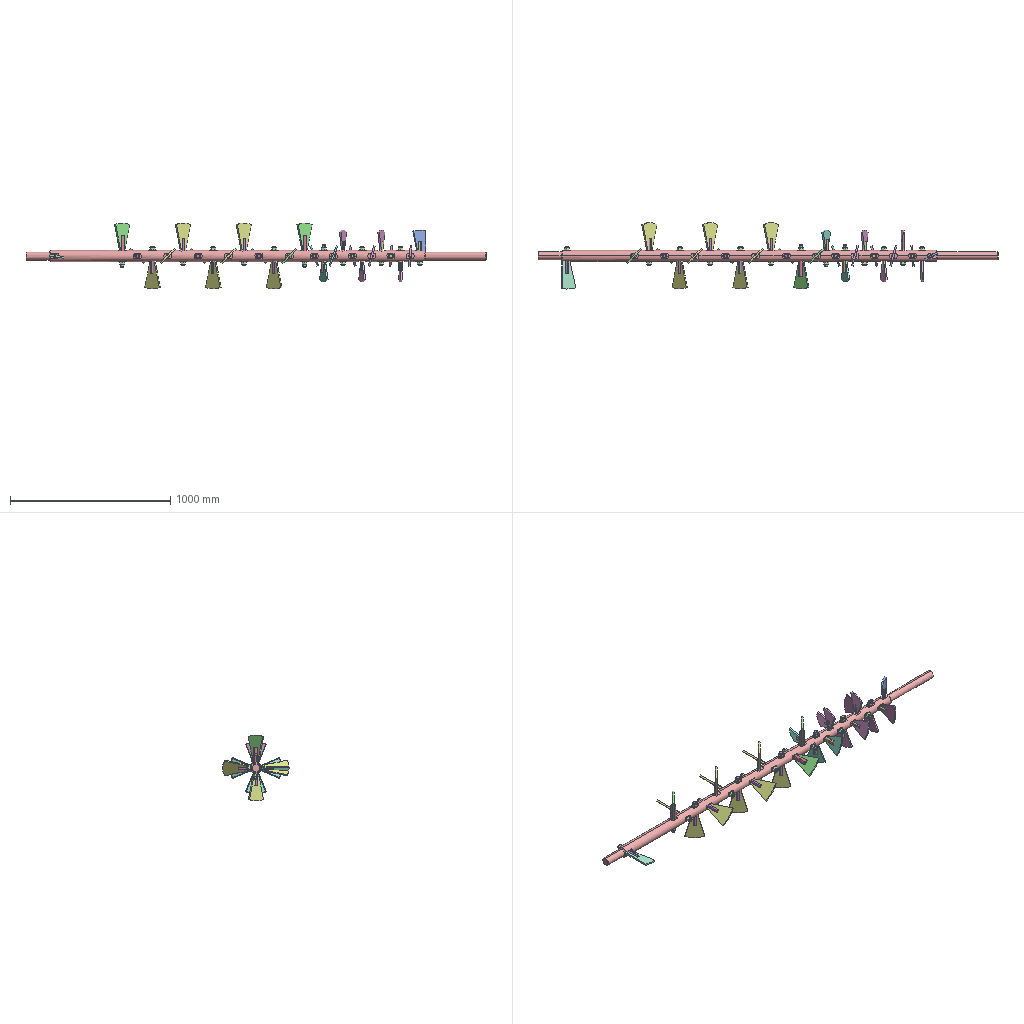Assembly | SolidWorks | 22 different items | 138 placed | box 2875 x 413 x 412 mm
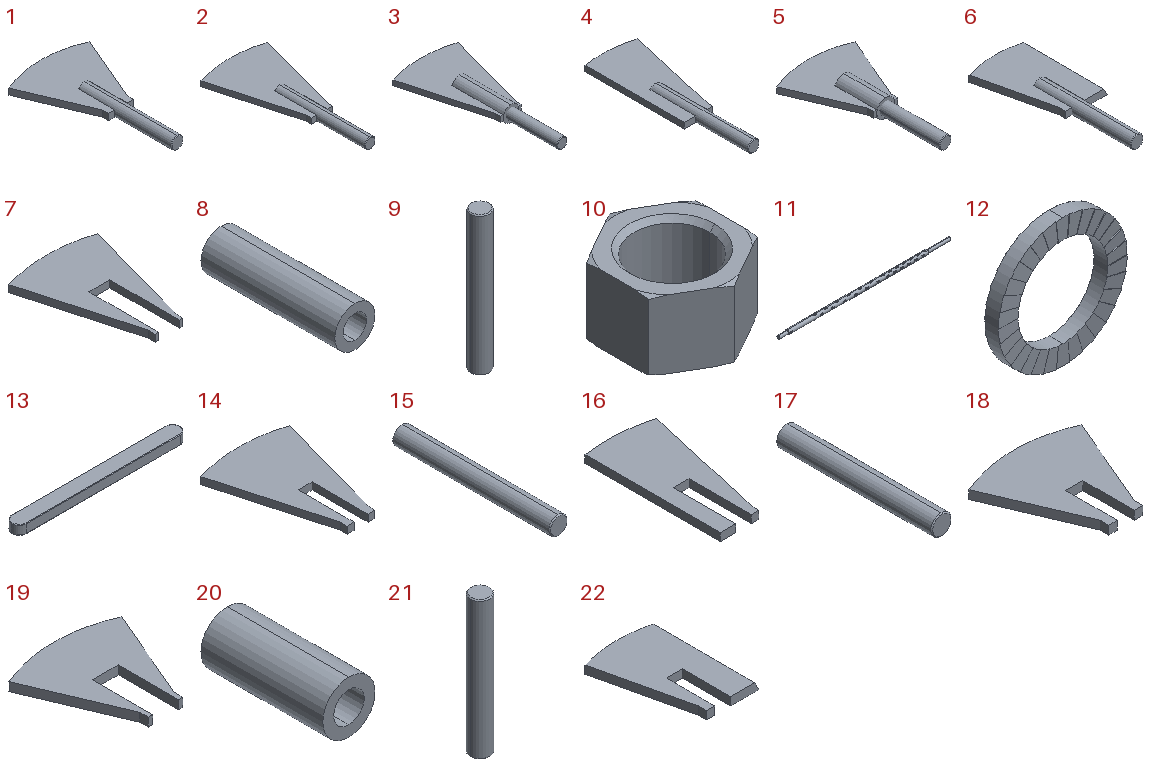Parts list (item | name | quantity | parent item | size | volume | features):
1 | (subassembly) | x8 | - | 130.916 x 223 x 20 mm | 143488 mm3 | -
2 | (subassembly) | x10 | - | 126.548 x 268 x 20 mm | 180390 mm3 | -
3 | (subassembly) | x3 | - | 126.548 x 276 x 30 mm | 214680 mm3 | -
4 | (subassembly) | x1 | - | 86.5 x 268 x 20 mm | 156047 mm3 | -
5 | (subassembly) | x3 | - | 130.202 x 230 x 30 mm | 165813 mm3 | -
6 | (subassembly) | x1 | - | 91.361 x 223 x 20 mm | 132533 mm3 | -
7 | - | x3 | in 3 | 126.548 x 176 x 10 mm | 112385 mm3 | features Extrusion 1, ICE 1
8 | - | x3 | in 3 | 30 x 100 x 30 mm | 55231 mm3 | features 3DProfileFeature 1, Extrusion 1, HoleWzd 1
9 | - | x3 | in 3 | 20 x 20 x 150 mm | 47063 mm3 | features Chamfer 1, Extrusion 1
10 | - | x26 | - | 28.6 x 32.95 x 18 mm | 6925 mm3 | features Cut 2, Chamfer 1, Extrusion 1
11 | - | x1 | - | 2875 x 70 x 70 mm | 9321994 mm3 | features ICE 18, MirrorPattern 7, LPattern 4, Fillet 2, Chamfer 1, Extrusion 1
12 | - | x26 | - | 30.7 x 3.4 x 30.7 mm | 1238 mm3 | features ICE 3, CirPattern 1, Extrusion 1, MirrorSolid 1
13 | - | x1 | - | 160 x 14 x 9 mm | 19730 mm3 | features Extrusion 1, Fillet 1
14 | - | x10 | in 2 | 126.548 x 176 x 10 mm | 126385 mm3 | features Extrusion 1, ICE 1
15 | - | x11 | in 2, 4 | 20 x 172 x 20 mm | 54005 mm3 | features Chamfer 1, Extrusion 1
16 | - | x1 | in 4 | 86.5 x 176 x 10 mm | 102042 mm3 | features Extrusion 1, ICE 1
17 | - | x9 | in 1, 6 | 20 x 152 x 20 mm | 47722 mm3 | features Chamfer 1, Extrusion 1
18 | - | x8 | in 1 | 130.916 x 131 x 10 mm | 95766 mm3 | features Extrusion 1, ICE 1
19 | - | x3 | in 5 | 130.202 x 130 x 10 mm | 85461 mm3 | features Extrusion 1
20 | - | x3 | in 5 | 30 x 70 x 30 mm | 36431 mm3 | features 3DProfileFeature 1, Extrusion 1, HoleWzd 1
21 | - | x3 | in 5 | 20 x 20 x 140 mm | 43922 mm3 | features Chamfer 1, Extrusion 1
22 | - | x1 | in 6 | 91.361 x 131 x 10 mm | 84811 mm3 | features ICE 2, Extrusion 1
Mates (type | each side: item.copy, entity, surface, feature):
In the top assembly
Concentric | 11.1 face cylinder Cut-Extrude11 | 17.1 face cylinder Boss-Extrude1
Coincident | 11.1 face plane Mirror3 | 18.1 face plane Boss-Extrude1
PlanarAngleDim | 1.1 plane | assembly plane
Concentric | 11.1 face cylinder LPattern1 | 17.2 face cylinder Boss-Extrude1
Coincident | 11.1 face plane LPattern1 | 18.2 face plane Boss-Extrude1
PlanarAngleDim | assembly plane | 1.2 plane
Concentric | 11.1 face cylinder LPattern1 | 17.3 face cylinder Boss-Extrude1
Coincident | 11.1 face plane LPattern1 | 18.3 face plane Boss-Extrude1
PlanarAngleDim | assembly plane | 1.3 plane
Concentric | 11.1 face cylinder LPattern1 | 17.4 face cylinder Boss-Extrude1
Coincident | 11.1 face plane LPattern1 | 18.4 face plane Boss-Extrude1
PlanarAngleDim | 1.4 plane | assembly plane
Concentric | 11.1 face cylinder Cut-Extrude9 | 17.5 face cylinder Boss-Extrude1
Coincident | 11.1 face plane Mirror2 | 18.5 face plane Boss-Extrude1
PlanarAngleDim | 1.5 plane | assembly plane
Concentric | 11.1 face cylinder LPattern2 | 17.6 face cylinder Boss-Extrude1
Coincident | 11.1 face plane LPattern2 | 18.6 face plane Boss-Extrude1
PlanarAngleDim | 1.6 plane | assembly plane
Concentric | 11.1 face cylinder LPattern2 | 17.7 face cylinder Boss-Extrude1
Coincident | 11.1 face plane LPattern2 | 18.7 face plane Boss-Extrude1
PlanarAngleDim | assembly plane | 1.7 plane
Concentric | 11.1 face cylinder LPattern2 | 17.8 face cylinder Boss-Extrude1
Coincident | 11.1 face plane LPattern2 | 18.8 face plane Boss-Extrude1
PlanarAngleDim | assembly plane | 1.8 plane
Concentric | 11.1 face cylinder Cut-Extrude15 | 20.1 face cylinder Boss-Extrude1
Coincident | 11.1 face plane Cut-Extrude14 | 20.1 face plane Boss-Extrude1
Concentric | 11.1 face cylinder LPattern1 | 20.2 face cylinder Boss-Extrude1
Coincident | 11.1 face plane LPattern1 | 19.1 face plane Boss-Extrude2
Concentric | 11.1 face cylinder LPattern2 | 20.3 face cylinder Boss-Extrude1
Coincident | 11.1 face plane LPattern2 | 20.3 face plane Boss-Extrude1
PlanarAngleDim | 5.1 plane | assembly plane
PlanarAngleDim | assembly plane | 5.2 plane
PlanarAngleDim | assembly plane | 5.3 plane
Concentric | 11.1 face cylinder Cut-Extrude13 | 8.1 face cylinder Boss-Extrude1
Coincident | 11.1 face plane Cut-Extrude12 | 7.1 face plane Boss-Extrude1
PlanarAngleDim | assembly plane | 3.1 plane
Concentric | 11.1 face cylinder Cut-Extrude19 | 8.2 face cylinder Boss-Extrude1
Coincident | 11.1 face plane Mirror7 | 8.2 face plane Boss-Extrude1
PlanarAngleDim | assembly plane | 3.2 plane
Concentric | 11.1 face cylinder LPattern3 | 15.1 face cylinder Boss-Extrude1
Coincident | 11.1 face plane LPattern3 | 14.1 face plane Boss-Extrude1
PlanarAngleDim | 2.1 plane | assembly plane
Concentric | 11.1 face cylinder LPattern4 | 15.2 face cylinder Boss-Extrude1
Coincident | 11.1 face plane LPattern4 | 14.2 face plane Boss-Extrude1
PlanarAngleDim | assembly plane | 2.2 plane
Concentric | 11.1 face cylinder LPattern3 | 15.3 face cylinder Boss-Extrude1
Coincident | 11.1 face plane LPattern3 | 14.3 face plane Boss-Extrude1
Parallel | 7.1 face plane Boss-Extrude1 | 14.3 face plane Boss-Extrude1
Concentric | 11.1 face cylinder LPattern4 | 15.4 face cylinder Boss-Extrude1
Coincident | 11.1 face plane LPattern4 | 14.4 face plane Boss-Extrude1
Parallel | 7.2 face plane Boss-Extrude1 | 14.4 face plane Boss-Extrude1
Concentric | 11.1 face cylinder LPattern3 | 15.5 face cylinder Boss-Extrude1
Coincident | 11.1 face plane LPattern3 | 14.5 face plane Boss-Extrude1
Parallel | 14.1 face plane Boss-Extrude1 | 14.5 face plane Boss-Extrude1
Concentric | 11.1 face cylinder LPattern4 | 15.6 face cylinder Boss-Extrude1
Coincident | 11.1 face plane LPattern4 | 14.6 face plane Boss-Extrude1
Parallel | 14.2 face plane Boss-Extrude1 | 14.6 face plane Boss-Extrude1
Concentric | 11.1 face cylinder LPattern3 | 15.7 face cylinder Boss-Extrude1
Coincident | 11.1 face plane LPattern3 | 14.7 face plane Boss-Extrude1
Parallel | 14.3 face plane Boss-Extrude1 | 14.7 face plane Boss-Extrude1
Concentric | 11.1 face cylinder LPattern4 | 15.8 face cylinder Boss-Extrude1
Coincident | 11.1 face plane LPattern4 | 14.8 face plane Boss-Extrude1
Parallel | 14.4 face plane Boss-Extrude1 | 14.8 face plane Boss-Extrude1
Concentric | 11.1 face cylinder LPattern3 | 15.9 face cylinder Boss-Extrude1
Coincident | 11.1 face plane LPattern3 | 14.9 face plane Boss-Extrude1
Parallel | 14.5 face plane Boss-Extrude1 | 14.9 face plane Boss-Extrude1
Concentric | 11.1 face cylinder LPattern4 | 15.10 face cylinder Boss-Extrude1
Coincident | 11.1 face plane LPattern4 | 14.10 face plane Boss-Extrude1
Parallel | 14.6 face plane Boss-Extrude1 | 14.10 face plane Boss-Extrude1
Concentric | 11.1 face cylinder LPattern3 | 8.3 face cylinder Boss-Extrude1
Coincident | 11.1 face plane LPattern3 | 8.3 face plane Boss-Extrude1
Parallel | 14.7 face plane Boss-Extrude1 | 7.3 face plane Boss-Extrude1
Concentric | 11.1 face cylinder Cut-Extrude7 | 17.9 face cylinder Boss-Extrude1
PlanarAngleDim | 6.1 plane | assembly plane
Concentric | 11.1 face cylinder Cut-Extrude17 | 15.11 face cylinder Boss-Extrude1
Coincident | 11.1 face plane Mirror6 | 16.1 face plane Boss-Extrude1
PlanarAngleDim | 4.1 plane | assembly plane
Coincident | 11.1 face plane Cut-Extrude6 | 22.1 face plane Boss-Extrude1
Concentric | 17.9 face cylinder Boss-Extrude1 | assembly face | 2 times
Concentric | 17.1 face cylinder Boss-Extrude1 | assembly face | 2 times
Concentric | 17.6 face cylinder Boss-Extrude1 | assembly face | 2 times
Concentric | 17.2 face cylinder Boss-Extrude1 | assembly face
Coincident | 11.1 face plane Cut-Extrude20 | 13.1 face plane Base-Extrude
Concentric | 11.1 face cylinder Cut-Extrude20 | 13.1 face cylinder Base-Extrude | 2 times
Concentric | 17.5 face cylinder Boss-Extrude1 | 12.1 face cylinder Boss-Extrude1
Concentric | 17.5 face cylinder Boss-Extrude1 | assembly face
Concentric | 17.1 face cylinder Boss-Extrude1 | 12.2 face cylinder Boss-Extrude1
Coincident | 11.1 face plane Cut-Extrude10 | 12.2 edge
Coincident | 12.2 edge | assembly face
Coincident | 11.1 face plane Cut-Extrude8 | 12.1 edge
Coincident | 12.1 edge | assembly face
Concentric | 17.6 face cylinder Boss-Extrude1 | 12.3 face cylinder Boss-Extrude1
Coincident | 11.1 face plane LPattern2 | 12.3 edge
Coincident | 12.3 edge | assembly face
Concentric | 17.9 face cylinder Boss-Extrude1 | 12.4 face cylinder Boss-Extrude1
Coincident | 11.1 face plane Mirror1 | 12.4 edge
Coincident | 12.4 edge | assembly face
Concentric | 9.1 face cylinder Boss-Extrude1 | 12.5 face cylinder Boss-Extrude1
Coincident | 11.1 face plane Cut-Extrude18 | 12.5 edge
Concentric | 9.1 face cylinder Boss-Extrude1 | assembly face
Coincident | 12.5 edge | assembly face
Concentric | 15.1 face cylinder Boss-Extrude1 | 12.6 face cylinder Boss-Extrude1
Coincident | 11.1 face plane LPattern3 | 12.6 edge
Concentric | 15.1 face cylinder Boss-Extrude1 | assembly face
Coincident | 12.6 edge | assembly face
Concentric | 15.2 face cylinder Boss-Extrude1 | 12.7 face cylinder Boss-Extrude1
Coincident | 11.1 face plane LPattern4 | 12.7 edge
Concentric | 15.2 face cylinder Boss-Extrude1 | assembly face
Coincident | 12.7 edge | assembly face
Concentric | 15.3 face cylinder Boss-Extrude1 | 12.8 face cylinder Boss-Extrude1
Coincident | 11.1 face plane LPattern3 | 12.8 edge
Concentric | 15.3 face cylinder Boss-Extrude1 | assembly face
Coincident | 12.8 edge | assembly face
Concentric | 15.11 face cylinder Boss-Extrude1 | 12.9 face cylinder Boss-Extrude1
Coincident | 11.1 face plane Cut-Extrude16 | 12.9 edge
Concentric | 15.11 face cylinder Boss-Extrude1 | assembly face
Coincident | 12.9 edge | assembly face
Concentric | 17.9 face cylinder Boss-Extrude1 | 10.1 face cylinder Base-Extrude
Coincident | 12.4 edge | 10.1 face plane Base-Extrude
Concentric | 17.5 face cylinder Boss-Extrude1 | 10.2 face cylinder Base-Extrude
Coincident | 12.1 edge | 10.2 face plane Base-Extrude
Concentric | 17.1 face cylinder Boss-Extrude1 | 10.3 face cylinder Base-Extrude
Coincident | 12.2 edge | 10.3 face plane Base-Extrude
Concentric | 17.6 face cylinder Boss-Extrude1 | 10.4 face cylinder Base-Extrude
Coincident | 12.3 edge | 10.4 face plane Base-Extrude
Concentric | 9.1 face cylinder Boss-Extrude1 | 10.5 face cylinder Base-Extrude
Coincident | 12.5 edge | 10.5 face plane Base-Extrude
Concentric | 15.1 face cylinder Boss-Extrude1 | 10.6 face cylinder Base-Extrude
Coincident | 12.6 edge | 10.6 face plane Base-Extrude
Concentric | 15.2 face cylinder Boss-Extrude1 | 10.7 face cylinder Base-Extrude
Coincident | 12.7 edge | 10.7 face plane Base-Extrude
Concentric | 15.3 face cylinder Boss-Extrude1 | 10.8 face cylinder Base-Extrude
Coincident | 12.8 edge | 10.8 face plane Base-Extrude
Concentric | 15.11 face cylinder Boss-Extrude1 | 10.9 face cylinder Base-Extrude
Coincident | 12.9 edge | 10.9 face plane Base-Extrude
In subassembly 2
Coincident | 14.11 plane | 15.12 plane | 2 times
Coincident | 14.11 face plane Cut-Extrude1 | 15.12 face plane Boss-Extrude1
In subassembly 3
Coincident | 7.4 face plane Cut-Extrude1 | 8.4 face plane Boss-Extrude1
Coincident | 7.4 plane | 8.4 plane | 2 times
Concentric | 8.4 face cylinder M20 Tapped Hole1 | 9.2 face cylinder Boss-Extrude1
Coincident | 8.4 plane | 9.2 face plane Boss-Extrude1
In subassembly 5
Coincident | 19.2 face plane Boss-Extrude2 | 20.4 face plane Boss-Extrude1
Coincident | 19.2 plane | 20.4 plane | 2 times
Concentric | 20.4 face cylinder M20 Tapped Hole1 | 21.1 face cylinder Boss-Extrude1
Coincident | 20.4 plane | 21.1 face plane Boss-Extrude1
In subassembly 4
Coincident | 16.2 face plane Cut-Extrude1 | 15.12 face plane Boss-Extrude1
Coincident | 16.2 plane | 15.12 plane | 2 times
In subassembly 1
Coincident | 18.9 face plane Cut-Extrude1 | 17.10 face plane Boss-Extrude1
Coincident | 18.9 plane | 17.10 plane | 2 times
In subassembly 6
Coincident | 22.2 plane | 17.10 plane | 2 times
Coincident | 22.2 face plane Cut-Extrude1 | 17.10 face plane Boss-Extrude1